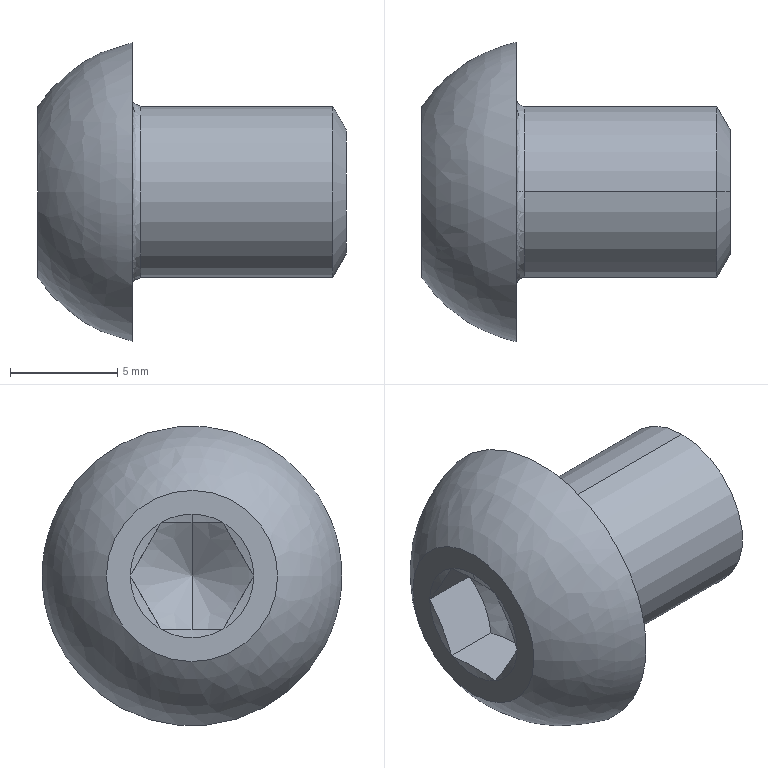Part | STEP file | 1 solid | 25 faces | box 14.4 x 14 x 14 mm | volume 924.643 mm3 | cone 11 | plane 9 | spline 3 | cylinder 2 | commonest cylinder face diameters 8 x2